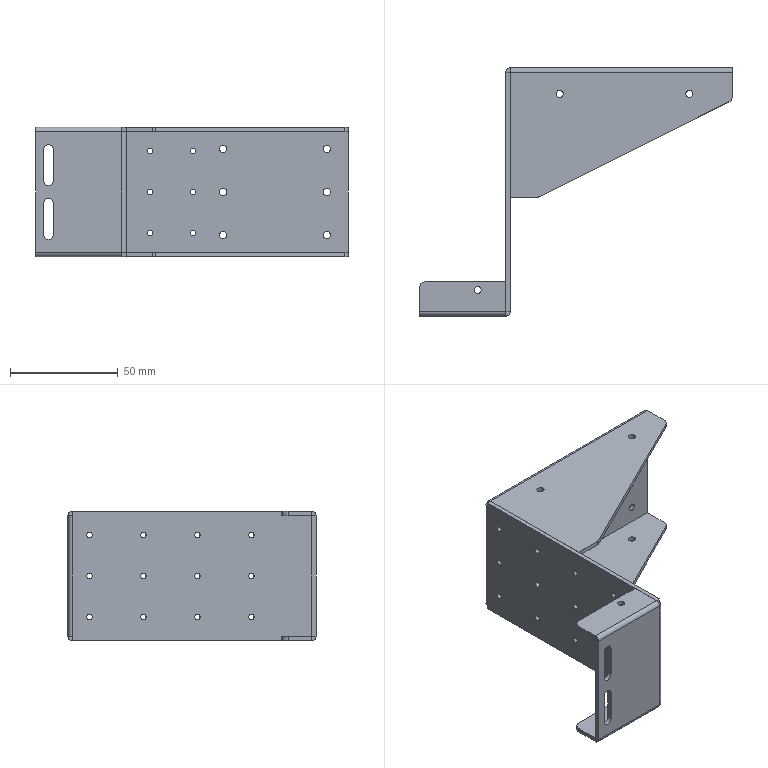Part | STEP file | 1 solid | 136 faces | box 145 x 115 x 60 mm | volume 47899 mm3 | cylinder 84 | plane 52 | commonest cylinder face diameters 2.5 x36 3.3 x24 0.02 x6 4.02 x6 4.5 x6 6 x6